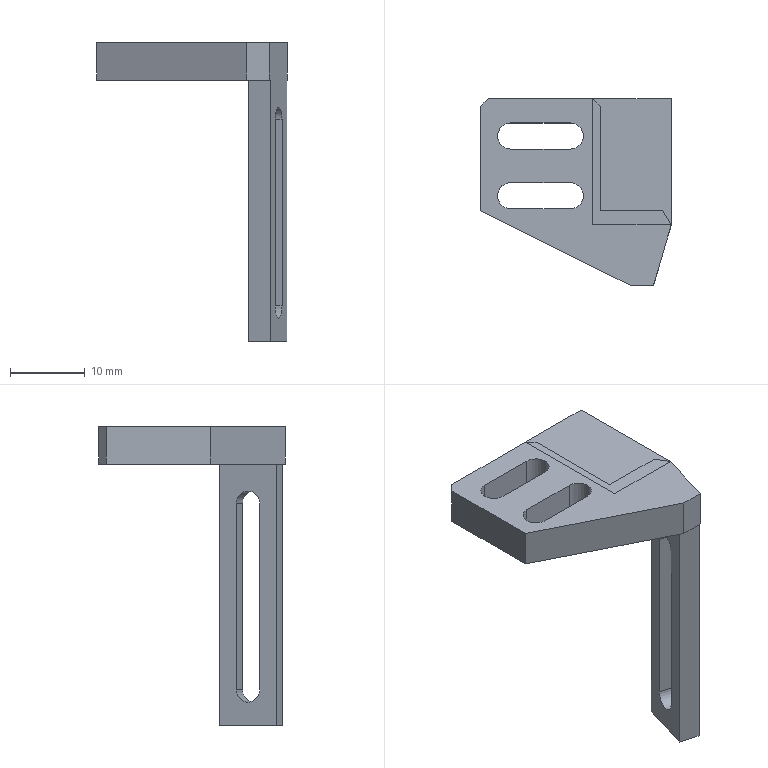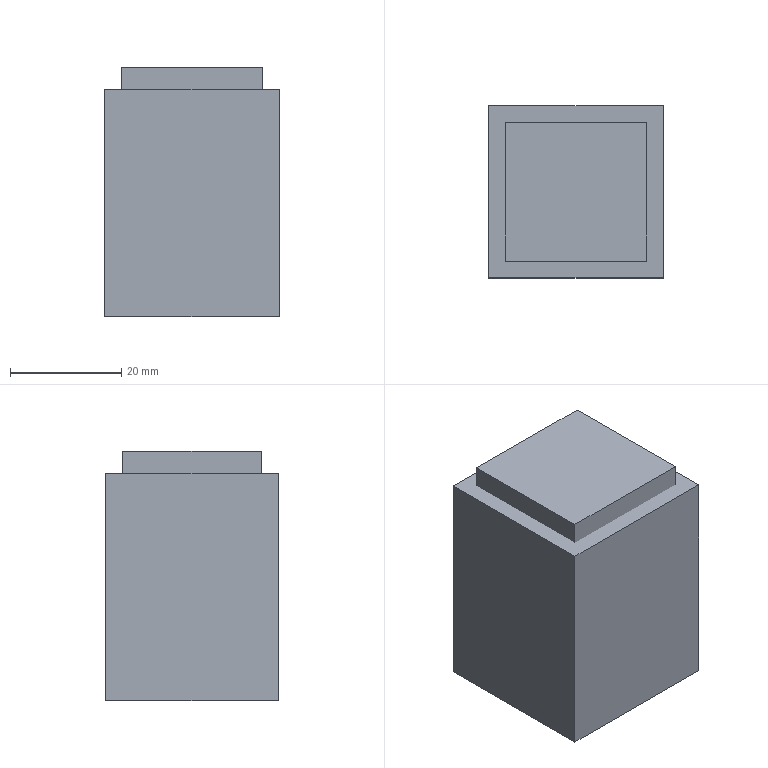CAM job | NX | 3+2 milling | part box 25.523 x 25 x 40 mm | stock box 31.523 x 31 x 45 mm
Tools:
number,name,description,diameter,corner_radius,flute_length,length,flutes
3,D63,Milling Tool-5 Parameters,63.0,0.0,50.0,75.0,2
4,D10,Milling Tool-5 Parameters,10.0,0.0,50.0,75.0,2
14,D10JING,Milling Tool-5 Parameters,10.0,0.0,50.0,75.0,2
1,D6A45,Milling Tool-5 Parameters,6.0,0.0,50.0,75.0,2
17,D3,Milling Tool-5 Parameters,3.0,0.0,50.0,75.0,2
7,D4R0.5,Milling Tool-5 Parameters,4.0,0.5,50.0,75.0,2
Operations:
program,operation,operation_type,tool,method,geometry_group,spindle_rpm,surface_speed,feed_per_tooth,feed_cut,feed_plunge,cut_length_mm,path_length_mm,cut_time_min,machine_time_min
1,FLOOR_WALL,VolumeBased25DMillingOperation,D63,METHOD,A,6500.0,1286.0,0.1154,1500.0,100.0,106.0,160.0,0.0707,0.0761
1,ADAPTIVE_MILLING,CavityMilling,D10,METHOD,A,7500.0,235.0,0.2,3000.0,1000.0,3790.143,4170.385,1.269,1.307
1,ZLEVEL_PROFILE,ZLevelMilling,D10JING,METHOD,A,7500.0,235.0,0.0667,1000.0,100.0,121.229,342.589,0.1212,0.1434
1,ZLEVEL_PROFILE_COPY,ZLevelMilling,D10JING,METHOD,A,7500.0,235.0,0.0667,1000.0,100.0,129.528,267.528,0.1295,0.1433
1,FLOOR_WALL_1_COPY_COPY,VolumeBased25DMillingOperation,D10JING,METHOD,A,7500.0,235.0,0.08,1200.0,1000.0,321.771,741.569,0.2718,0.3138
1,PLANAR_MILL,PlanarMilling,D6A45,METHOD,A,7500.0,141.0,0.0833,1250.0,100.0,33.26,91.26,0.0266,0.0324
1,PLANAR_MILL_COPY,PlanarMilling,D6A45,METHOD,A,7500.0,141.0,0.0833,1250.0,100.0,84.658,212.658,0.0677,0.0805
2,FLOOR_WALL_COPY,VolumeBased25DMillingOperation,D63,METHOD,B,6500.0,1286.0,0.1154,1500.0,100.0,500.0,1126.001,0.3333,0.3959
2,ZLEVEL_PROFILE_1,ZLevelMilling,D3,METHOD,B,7500.0,70.0,0.08,1200.0,1000.0,948.107,1082.152,0.7977,0.8111
2,PLANAR_MILL_COPY_1,PlanarMilling,D6A45,METHOD,B,7500.0,141.0,0.0833,1250.0,100.0,156.346,352.886,0.1251,0.1447
3,ZLEVEL_PROFILE_1_COPY,ZLevelMilling,D3,METHOD,C,7500.0,70.0,0.08,1200.0,1000.0,799.548,860.548,0.6701,0.6762
3,PLANAR_MILL_COPY_1_COPY,PlanarMilling,D6A45,METHOD,C,7500.0,141.0,0.0833,1250.0,100.0,65.312,123.312,0.0522,0.058
4,FLOOR_WALL_1,VolumeBased25DMillingOperation,D10,METHOD,D,7500.0,0.0,0.0,2000.0,100.0,498.0,664.56,0.249,0.2657
4,FLOOR_WALL_1_COPY_COPY_COPY,VolumeBased25DMillingOperation,D10JING,METHOD,D,7500.0,235.0,0.08,1200.0,1000.0,95.6,262.769,0.0817,0.0984
4,PLANAR_MILL_COPY_1_COPY_1,PlanarMilling,D6A45,METHOD,D,7500.0,141.0,0.0833,1250.0,100.0,21.491,184.134,0.0172,0.0335
4,ZLEVEL_PROFILE_1_1,ZLevelMilling,D4R0.5,METHOD,D,7500.0,94.0,0.1667,2500.0,1000.0,315.482,375.209,0.1274,0.1334